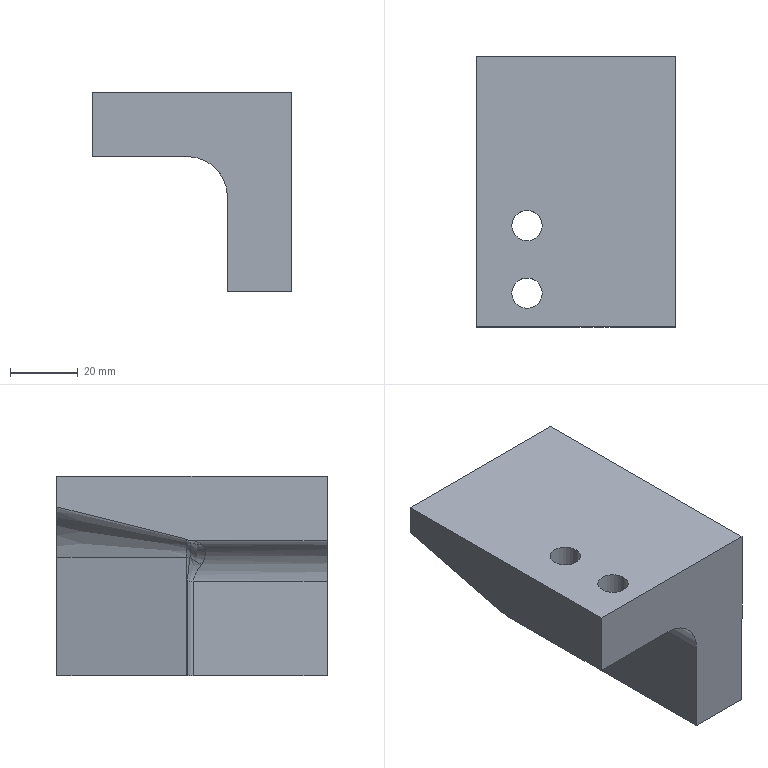Part | 1 solid | 30 faces | box 59 x 80 x 59 mm | volume 130851 mm3 | cylinder 13 | plane 12 | spline 4 | cone 1 | commonest cylinder face diameters 9 x4 15 x4 4 x2 10 x2 24 x1
STEP:
#1=CARTESIAN_POINT('',(-105.5,-10.,19.));
#2=VERTEX_POINT('',#1);
#3=CARTESIAN_POINT('',(-120.5,-10.,19.));
#4=VERTEX_POINT('',#3);
#5=CARTESIAN_POINT('',(-113.,-10.,19.));
#6=DIRECTION('',(0.,0.,1.));
#7=DIRECTION('',(1.,0.,0.));
#8=AXIS2_PLACEMENT_3D('',#5,#6,#7);
#9=CIRCLE('',#8,7.5);
#10=EDGE_CURVE('',#2,#4,#9,.T.);
#11=ORIENTED_EDGE('',*,*,#10,.T.);
#12=CARTESIAN_POINT('',(-120.5,-10.,10.));
#13=VERTEX_POINT('',#12);
#14=CARTESIAN_POINT('',(-120.5,-10.,10.));
#15=DIRECTION('',(0.,0.,-1.));
#16=VECTOR('',#15,1000.);
#17=LINE('',#14,#16);
#18=EDGE_CURVE('',#4,#13,#17,.T.);
#19=ORIENTED_EDGE('',*,*,#18,.T.);
#20=CARTESIAN_POINT('',(-105.5,-10.,10.));
#21=VERTEX_POINT('',#20);
#22=CARTESIAN_POINT('',(-113.,-10.,10.));
#23=DIRECTION('',(0.,0.,1.));
#24=DIRECTION('',(1.,0.,0.));
#25=AXIS2_PLACEMENT_3D('',#22,#23,#24);
#26=CIRCLE('',#25,7.5);
#27=EDGE_CURVE('',#21,#13,#26,.T.);
#28=ORIENTED_EDGE('',*,*,#27,.F.);
#29=CARTESIAN_POINT('',(-105.5,-10.,10.));
#30=DIRECTION('',(0.,0.,-1.));
#31=VECTOR('',#30,1000.);
#32=LINE('',#29,#31);
#33=EDGE_CURVE('',#2,#21,#32,.T.);
#34=ORIENTED_EDGE('',*,*,#33,.F.);
#35=EDGE_LOOP('',(#11,#19,#28,#34));
#36=FACE_OUTER_BOUND('',#35,.T.);
#37=CARTESIAN_POINT('',(-113.,-10.,10.));
#38=DIRECTION('',(0.,0.,-1.));
#39=DIRECTION('',(1.,0.,0.));
#40=AXIS2_PLACEMENT_3D('',#37,#38,#39);
#41=CYLINDRICAL_SURFACE('',#40,7.5);
#42=ADVANCED_FACE('',(#36),#41,.F.);
#43=CARTESIAN_POINT('',(-105.5,-30.,19.));
#44=VERTEX_POINT('',#43);
#45=CARTESIAN_POINT('',(-120.5,-30.,19.));
#46=VERTEX_POINT('',#45);
#47=CARTESIAN_POINT('',(-113.,-30.,19.));
#48=DIRECTION('',(0.,0.,1.));
#49=DIRECTION('',(1.,0.,0.));
#50=AXIS2_PLACEMENT_3D('',#47,#48,#49);
#51=CIRCLE('',#50,7.5);
#52=EDGE_CURVE('',#44,#46,#51,.T.);
#53=ORIENTED_EDGE('',*,*,#52,.T.);
#54=CARTESIAN_POINT('',(-120.5,-30.,10.));
#55=VERTEX_POINT('',#54);
#56=CARTESIAN_POINT('',(-120.5,-30.,10.));
#57=DIRECTION('',(0.,0.,-1.));
#58=VECTOR('',#57,1000.);
#59=LINE('',#56,#58);
#60=EDGE_CURVE('',#46,#55,#59,.T.);
#61=ORIENTED_EDGE('',*,*,#60,.T.);
#62=CARTESIAN_POINT('',(-105.5,-30.,10.));
#63=VERTEX_POINT('',#62);
#64=CARTESIAN_POINT('',(-113.,-30.,10.));
#65=DIRECTION('',(0.,0.,1.));
#66=DIRECTION('',(1.,0.,0.));
#67=AXIS2_PLACEMENT_3D('',#64,#65,#66);
#68=CIRCLE('',#67,7.5);
#69=EDGE_CURVE('',#63,#55,#68,.T.);
#70=ORIENTED_EDGE('',*,*,#69,.F.);
#71=CARTESIAN_POINT('',(-105.5,-30.,10.));
#72=DIRECTION('',(0.,0.,-1.));
#73=VECTOR('',#72,1000.);
#74=LINE('',#71,#73);
#75=EDGE_CURVE('',#44,#63,#74,.T.);
#76=ORIENTED_EDGE('',*,*,#75,.F.);
#77=EDGE_LOOP('',(#53,#61,#70,#76));
#78=FACE_OUTER_BOUND('',#77,.T.);
#79=CARTESIAN_POINT('',(-113.,-30.,10.));
#80=DIRECTION('',(0.,0.,-1.));
#81=DIRECTION('',(1.,0.,0.));
#82=AXIS2_PLACEMENT_3D('',#79,#80,#81);
#83=CYLINDRICAL_SURFACE('',#82,7.5);
#84=ADVANCED_FACE('',(#78),#83,.F.);
#85=CARTESIAN_POINT('',(-108.5,-10.,29.));
#86=VERTEX_POINT('',#85);
#87=CARTESIAN_POINT('',(-117.5,-10.,29.));
#88=VERTEX_POINT('',#87);
#89=CARTESIAN_POINT('',(-113.,-10.,29.));
#90=DIRECTION('',(0.,0.,1.));
#91=DIRECTION('',(-1.,0.,0.));
#92=AXIS2_PLACEMENT_3D('',#89,#90,#91);
#93=CIRCLE('',#92,4.5);
#94=EDGE_CURVE('',#86,#88,#93,.T.);
#95=ORIENTED_EDGE('',*,*,#94,.T.);
#96=CARTESIAN_POINT('',(-117.5,-10.,19.));
#97=VERTEX_POINT('',#96);
#98=CARTESIAN_POINT('',(-117.5,-10.,10.));
#99=DIRECTION('',(0.,0.,-1.));
#100=VECTOR('',#99,1000.);
#101=LINE('',#98,#100);
#102=EDGE_CURVE('',#88,#97,#101,.T.);
#103=ORIENTED_EDGE('',*,*,#102,.T.);
#104=CARTESIAN_POINT('',(-108.5,-10.,19.));
#105=VERTEX_POINT('',#104);
#106=CARTESIAN_POINT('',(-113.,-10.,19.));
#107=DIRECTION('',(0.,0.,1.));
#108=DIRECTION('',(1.,0.,0.));
#109=AXIS2_PLACEMENT_3D('',#106,#107,#108);
#110=CIRCLE('',#109,4.5);
#111=EDGE_CURVE('',#105,#97,#110,.T.);
#112=ORIENTED_EDGE('',*,*,#111,.F.);
#113=CARTESIAN_POINT('',(-108.5,-10.,10.));
#114=DIRECTION('',(0.,0.,-1.));
#115=VECTOR('',#114,1000.);
#116=LINE('',#113,#115);
#117=EDGE_CURVE('',#86,#105,#116,.T.);
#118=ORIENTED_EDGE('',*,*,#117,.F.);
#119=EDGE_LOOP('',(#95,#103,#112,#118));
#120=FACE_OUTER_BOUND('',#119,.T.);
#121=CARTESIAN_POINT('',(-113.,-10.,10.));
#122=DIRECTION('',(0.,0.,-1.));
#123=DIRECTION('',(1.,0.,0.));
#124=AXIS2_PLACEMENT_3D('',#121,#122,#123);
#125=CYLINDRICAL_SURFACE('',#124,4.5);
#126=ADVANCED_FACE('',(#120),#125,.F.);
#127=CARTESIAN_POINT('',(-108.5,-30.,29.));
#128=VERTEX_POINT('',#127);
#129=CARTESIAN_POINT('',(-117.5,-30.,29.));
#130=VERTEX_POINT('',#129);
#131=CARTESIAN_POINT('',(-113.,-30.,29.));
#132=DIRECTION('',(0.,0.,1.));
#133=DIRECTION('',(-1.,0.,0.));
#134=AXIS2_PLACEMENT_3D('',#131,#132,#133);
#135=CIRCLE('',#134,4.5);
#136=EDGE_CURVE('',#128,#130,#135,.T.);
#137=ORIENTED_EDGE('',*,*,#136,.T.);
#138=CARTESIAN_POINT('',(-117.5,-30.,19.));
#139=VERTEX_POINT('',#138);
#140=CARTESIAN_POINT('',(-117.5,-30.,10.));
#141=DIRECTION('',(0.,0.,-1.));
#142=VECTOR('',#141,1000.);
#143=LINE('',#140,#142);
#144=EDGE_CURVE('',#130,#139,#143,.T.);
#145=ORIENTED_EDGE('',*,*,#144,.T.);
#146=CARTESIAN_POINT('',(-108.5,-30.,19.));
#147=VERTEX_POINT('',#146);
#148=CARTESIAN_POINT('',(-113.,-30.,19.));
#149=DIRECTION('',(0.,0.,1.));
#150=DIRECTION('',(1.,0.,0.));
#151=AXIS2_PLACEMENT_3D('',#148,#149,#150);
#152=CIRCLE('',#151,4.5);
#153=EDGE_CURVE('',#147,#139,#152,.T.);
#154=ORIENTED_EDGE('',*,*,#153,.F.);
#155=CARTESIAN_POINT('',(-108.5,-30.,10.));
#156=DIRECTION('',(0.,0.,-1.));
#157=VECTOR('',#156,1000.);
#158=LINE('',#155,#157);
#159=EDGE_CURVE('',#128,#147,#158,.T.);
#160=ORIENTED_EDGE('',*,*,#159,.F.);
#161=EDGE_LOOP('',(#137,#145,#154,#160));
#162=FACE_OUTER_BOUND('',#161,.T.);
#163=CARTESIAN_POINT('',(-113.,-30.,10.));
#164=DIRECTION('',(0.,0.,-1.));
#165=DIRECTION('',(1.,0.,0.));
#166=AXIS2_PLACEMENT_3D('',#163,#164,#165);
#167=CYLINDRICAL_SURFACE('',#166,4.5);
#168=ADVANCED_FACE('',(#162),#167,.F.);
#169=CARTESIAN_POINT('',(-69.,40.,29.));
#170=VERTEX_POINT('',#169);
#171=CARTESIAN_POINT('',(-69.,40.,-30.));
#172=VERTEX_POINT('',#171);
#173=CARTESIAN_POINT('',(-69.,40.,-30.));
#174=DIRECTION('',(0.,0.,-1.));
#175=VECTOR('',#174,1000.);
#176=LINE('',#173,#175);
#177=EDGE_CURVE('',#170,#172,#176,.T.);
#178=ORIENTED_EDGE('',*,*,#177,.T.);
#179=CARTESIAN_POINT('',(-78.,40.,-30.));
#180=VERTEX_POINT('',#179);
#181=CARTESIAN_POINT('',(-88.,40.,-30.));
#182=DIRECTION('',(1.,0.,0.));
#183=VECTOR('',#182,1000.);
#184=LINE('',#181,#183);
#185=EDGE_CURVE('',#180,#172,#184,.T.);
#186=ORIENTED_EDGE('',*,*,#185,.F.);
#187=CARTESIAN_POINT('',(-78.,40.,5.));
#188=VERTEX_POINT('',#187);
#189=CARTESIAN_POINT('',(-78.,40.,5.));
#190=DIRECTION('',(0.,0.,-1.));
#191=VECTOR('',#190,1000.);
#192=LINE('',#189,#191);
#193=EDGE_CURVE('',#188,#180,#192,.T.);
#194=ORIENTED_EDGE('',*,*,#193,.F.);
#195=CARTESIAN_POINT('',(-93.,40.,20.));
#196=VERTEX_POINT('',#195);
#197=CARTESIAN_POINT('',(-93.,40.,5.));
#198=DIRECTION('',(0.,1.,0.));
#199=DIRECTION('',(0.,0.,1.));
#200=AXIS2_PLACEMENT_3D('',#197,#198,#199);
#201=CIRCLE('',#200,15.);
#202=EDGE_CURVE('',#196,#188,#201,.T.);
#203=ORIENTED_EDGE('',*,*,#202,.F.);
#204=CARTESIAN_POINT('',(-128.,40.,20.));
#205=VERTEX_POINT('',#204);
#206=CARTESIAN_POINT('',(-133.,40.,20.));
#207=DIRECTION('',(1.,0.,0.));
#208=VECTOR('',#207,1000.);
#209=LINE('',#206,#208);
#210=EDGE_CURVE('',#205,#196,#209,.T.);
#211=ORIENTED_EDGE('',*,*,#210,.F.);
#212=CARTESIAN_POINT('',(-128.,40.,29.));
#213=VERTEX_POINT('',#212);
#214=CARTESIAN_POINT('',(-128.,40.,30.));
#215=DIRECTION('',(0.,0.,-1.));
#216=VECTOR('',#215,1000.);
#217=LINE('',#214,#216);
#218=EDGE_CURVE('',#213,#205,#217,.T.);
#219=ORIENTED_EDGE('',*,*,#218,.F.);
#220=CARTESIAN_POINT('',(-68.,40.,29.));
#221=DIRECTION('',(1.,0.,0.));
#222=VECTOR('',#221,1000.);
#223=LINE('',#220,#222);
#224=EDGE_CURVE('',#213,#170,#223,.T.);
#225=ORIENTED_EDGE('',*,*,#224,.T.);
#226=EDGE_LOOP('',(#178,#186,#194,#203,#211,#219,#225));
#227=FACE_OUTER_BOUND('',#226,.T.);
#228=CARTESIAN_POINT('',(-100.,40.,-2.));
#229=DIRECTION('',(0.,-1.,0.));
#230=DIRECTION('',(0.,0.,-1.));
#231=AXIS2_PLACEMENT_3D('',#228,#229,#230);
#232=PLANE('',#231);
#233=ADVANCED_FACE('',(#227),#232,.F.);
#234=CARTESIAN_POINT('',(-69.,-40.,29.));
#235=VERTEX_POINT('',#234);
#236=CARTESIAN_POINT('',(-128.,-40.,29.));
#237=VERTEX_POINT('',#236);
#238=CARTESIAN_POINT('',(-68.,-40.,29.));
#239=DIRECTION('',(-1.,0.,0.));
#240=VECTOR('',#239,1000.);
#241=LINE('',#238,#240);
#242=EDGE_CURVE('',#235,#237,#241,.T.);
#243=ORIENTED_EDGE('',*,*,#242,.T.);
#244=CARTESIAN_POINT('',(-128.,-40.,10.));
#245=VERTEX_POINT('',#244);
#246=CARTESIAN_POINT('',(-128.,-40.,30.));
#247=DIRECTION('',(0.,0.,-1.));
#248=VECTOR('',#247,1000.);
#249=LINE('',#246,#248);
#250=EDGE_CURVE('',#237,#245,#249,.T.);
#251=ORIENTED_EDGE('',*,*,#250,.T.);
#252=CARTESIAN_POINT('',(-100.,-40.,10.));
#253=VERTEX_POINT('',#252);
#254=CARTESIAN_POINT('',(-128.,-40.,10.));
#255=DIRECTION('',(1.,0.,0.));
#256=VECTOR('',#255,1000.);
#257=LINE('',#254,#256);
#258=EDGE_CURVE('',#245,#253,#257,.T.);
#259=ORIENTED_EDGE('',*,*,#258,.T.);
#260=CARTESIAN_POINT('',(-88.,-40.,-2.));
#261=VERTEX_POINT('',#260);
#262=CARTESIAN_POINT('',(-100.,-40.,-2.));
#263=DIRECTION('',(0.,1.,0.));
#264=DIRECTION('',(0.,0.,-1.));
#265=AXIS2_PLACEMENT_3D('',#262,#263,#264);
#266=CIRCLE('',#265,12.);
#267=EDGE_CURVE('',#253,#261,#266,.T.);
#268=ORIENTED_EDGE('',*,*,#267,.T.);
#269=CARTESIAN_POINT('',(-88.,-40.,-30.));
#270=VERTEX_POINT('',#269);
#271=CARTESIAN_POINT('',(-88.,-40.,-2.));
#272=DIRECTION('',(0.,0.,-1.));
#273=VECTOR('',#272,1000.);
#274=LINE('',#271,#273);
#275=EDGE_CURVE('',#261,#270,#274,.T.);
#276=ORIENTED_EDGE('',*,*,#275,.T.);
#277=CARTESIAN_POINT('',(-69.,-40.,-30.));
#278=VERTEX_POINT('',#277);
#279=CARTESIAN_POINT('',(-88.,-40.,-30.));
#280=DIRECTION('',(1.,0.,0.));
#281=VECTOR('',#280,1000.);
#282=LINE('',#279,#281);
#283=EDGE_CURVE('',#270,#278,#282,.T.);
#284=ORIENTED_EDGE('',*,*,#283,.T.);
#285=CARTESIAN_POINT('',(-69.,-40.,-30.));
#286=DIRECTION('',(0.,0.,1.));
#287=VECTOR('',#286,1000.);
#288=LINE('',#285,#287);
#289=EDGE_CURVE('',#278,#235,#288,.T.);
#290=ORIENTED_EDGE('',*,*,#289,.T.);
#291=EDGE_LOOP('',(#243,#251,#259,#268,#276,#284,#290));
#292=FACE_OUTER_BOUND('',#291,.T.);
#293=CARTESIAN_POINT('',(-100.,-40.,-2.));
#294=DIRECTION('',(0.,-1.,0.));
#295=DIRECTION('',(0.,0.,-1.));
#296=AXIS2_PLACEMENT_3D('',#293,#294,#295);
#297=PLANE('',#296);
#298=ADVANCED_FACE('',(#292),#297,.T.);
#299=CARTESIAN_POINT('',(-87.621,1.515,-30.));
#300=VERTEX_POINT('',#299);
#301=CARTESIAN_POINT('',(-87.687,1.303,-30.));
#302=VERTEX_POINT('',#301);
#303=CARTESIAN_POINT('',(-89.562,2.,-30.));
#304=DIRECTION('',(0.,0.,-1.));
#305=DIRECTION('',(-1.,0.,0.));
#306=AXIS2_PLACEMENT_3D('',#303,#304,#305);
#307=CIRCLE('',#306,2.);
#308=EDGE_CURVE('',#300,#302,#307,.T.);
#309=ORIENTED_EDGE('',*,*,#308,.F.);
#310=CARTESIAN_POINT('',(-78.,40.,-30.));
#311=DIRECTION('',(-0.2425,-0.9701,0.));
#312=VECTOR('',#311,1000.);
#313=LINE('',#310,#312);
#314=EDGE_CURVE('',#180,#300,#313,.T.);
#315=ORIENTED_EDGE('',*,*,#314,.F.);
#316=ORIENTED_EDGE('',*,*,#185,.T.);
#317=CARTESIAN_POINT('',(-69.,40.,-30.));
#318=DIRECTION('',(0.,-1.,0.));
#319=VECTOR('',#318,1000.);
#320=LINE('',#317,#319);
#321=EDGE_CURVE('',#172,#278,#320,.T.);
#322=ORIENTED_EDGE('',*,*,#321,.T.);
#323=ORIENTED_EDGE('',*,*,#283,.F.);
#324=CARTESIAN_POINT('',(-88.,-0.4384,-30.));
#325=VERTEX_POINT('',#324);
#326=CARTESIAN_POINT('',(-88.,40.,-30.));
#327=DIRECTION('',(0.,-1.,0.));
#328=VECTOR('',#327,1000.);
#329=LINE('',#326,#328);
#330=EDGE_CURVE('',#325,#270,#329,.T.);
#331=ORIENTED_EDGE('',*,*,#330,.F.);
#332=CARTESIAN_POINT('',(-83.,-0.4384,-30.));
#333=DIRECTION('',(0.,0.,1.));
#334=DIRECTION('',(-1.,0.,0.));
#335=AXIS2_PLACEMENT_3D('',#332,#333,#334);
#336=CIRCLE('',#335,5.);
#337=EDGE_CURVE('',#302,#325,#336,.T.);
#338=ORIENTED_EDGE('',*,*,#337,.F.);
#339=EDGE_LOOP('',(#309,#315,#316,#322,#323,#331,#338));
#340=FACE_OUTER_BOUND('',#339,.T.);
#341=CARTESIAN_POINT('',(-88.,40.,-30.));
#342=DIRECTION('',(0.,0.,1.));
#343=DIRECTION('',(-1.,0.,0.));
#344=AXIS2_PLACEMENT_3D('',#341,#342,#343);
#345=PLANE('',#344);
#346=ADVANCED_FACE('',(#340),#345,.F.);
#347=ORIENTED_EDGE('',*,*,#94,.F.);
#348=CARTESIAN_POINT('',(-113.,-10.,29.));
#349=DIRECTION('',(0.,0.,1.));
#350=DIRECTION('',(-1.,0.,0.));
#351=AXIS2_PLACEMENT_3D('',#348,#349,#350);
#352=CIRCLE('',#351,4.5);
#353=EDGE_CURVE('',#88,#86,#352,.T.);
#354=ORIENTED_EDGE('',*,*,#353,.F.);
#355=EDGE_LOOP('',(#347,#354));
#356=FACE_BOUND('',#355,.T.);
#357=ORIENTED_EDGE('',*,*,#136,.F.);
#358=CARTESIAN_POINT('',(-113.,-30.,29.));
#359=DIRECTION('',(0.,0.,1.));
#360=DIRECTION('',(-1.,0.,0.));
#361=AXIS2_PLACEMENT_3D('',#358,#359,#360);
#362=CIRCLE('',#361,4.5);
#363=EDGE_CURVE('',#130,#128,#362,.T.);
#364=ORIENTED_EDGE('',*,*,#363,.F.);
#365=EDGE_LOOP('',(#357,#364));
#366=FACE_BOUND('',#365,.T.);
#367=ORIENTED_EDGE('',*,*,#224,.F.);
#368=CARTESIAN_POINT('',(-128.,40.,29.));
#369=DIRECTION('',(0.,1.,0.));
#370=VECTOR('',#369,1000.);
#371=LINE('',#368,#370);
#372=EDGE_CURVE('',#237,#213,#371,.T.);
#373=ORIENTED_EDGE('',*,*,#372,.F.);
#374=ORIENTED_EDGE('',*,*,#242,.F.);
#375=CARTESIAN_POINT('',(-69.,40.,29.));
#376=DIRECTION('',(0.,1.,0.));
#377=VECTOR('',#376,1000.);
#378=LINE('',#375,#377);
#379=EDGE_CURVE('',#235,#170,#378,.T.);
#380=ORIENTED_EDGE('',*,*,#379,.T.);
#381=EDGE_LOOP('',(#367,#373,#374,#380));
#382=FACE_OUTER_BOUND('',#381,.T.);
#383=CARTESIAN_POINT('',(-98.,0.,29.));
#384=DIRECTION('',(0.,0.,1.));
#385=DIRECTION('',(-1.,0.,0.));
#386=AXIS2_PLACEMENT_3D('',#383,#384,#385);
#387=PLANE('',#386);
#388=ADVANCED_FACE('',(#356,#366,#382),#387,.T.);
#389=CARTESIAN_POINT('',(-128.,-0.4384,10.));
#390=VERTEX_POINT('',#389);
#391=CARTESIAN_POINT('',(-128.,40.,10.));
#392=DIRECTION('',(0.,-1.,0.));
#393=VECTOR('',#392,1000.);
#394=LINE('',#391,#393);
#395=EDGE_CURVE('',#390,#245,#394,.T.);
#396=ORIENTED_EDGE('',*,*,#395,.T.);
#397=ORIENTED_EDGE('',*,*,#250,.F.);
#398=ORIENTED_EDGE('',*,*,#372,.T.);
#399=ORIENTED_EDGE('',*,*,#218,.T.);
#400=CARTESIAN_POINT('',(-128.,1.515,10.379));
#401=VERTEX_POINT('',#400);
#402=CARTESIAN_POINT('',(-128.,40.,20.));
#403=DIRECTION('',(0.,0.9701,0.2425));
#404=VECTOR('',#403,1000.);
#405=LINE('',#402,#404);
#406=EDGE_CURVE('',#401,#205,#405,.T.);
#407=ORIENTED_EDGE('',*,*,#406,.F.);
#408=CARTESIAN_POINT('',(-128.,1.303,10.313));
#409=VERTEX_POINT('',#408);
#410=CARTESIAN_POINT('',(-128.,2.,8.438));
#411=DIRECTION('',(-1.,0.,0.));
#412=DIRECTION('',(0.,0.,1.));
#413=AXIS2_PLACEMENT_3D('',#410,#411,#412);
#414=CIRCLE('',#413,2.);
#415=EDGE_CURVE('',#409,#401,#414,.T.);
#416=ORIENTED_EDGE('',*,*,#415,.F.);
#417=CARTESIAN_POINT('',(-128.,-0.4384,15.));
#418=DIRECTION('',(1.,0.,0.));
#419=DIRECTION('',(0.,0.,1.));
#420=AXIS2_PLACEMENT_3D('',#417,#418,#419);
#421=CIRCLE('',#420,5.);
#422=EDGE_CURVE('',#390,#409,#421,.T.);
#423=ORIENTED_EDGE('',*,*,#422,.F.);
#424=EDGE_LOOP('',(#396,#397,#398,#399,#407,#416,#423));
#425=FACE_OUTER_BOUND('',#424,.T.);
#426=CARTESIAN_POINT('',(-128.,40.,30.));
#427=DIRECTION('',(1.,0.,0.));
#428=DIRECTION('',(0.,0.,1.));
#429=AXIS2_PLACEMENT_3D('',#426,#427,#428);
#430=PLANE('',#429);
#431=ADVANCED_FACE('',(#425),#430,.F.);
#432=ORIENTED_EDGE('',*,*,#144,.F.);
#433=ORIENTED_EDGE('',*,*,#363,.T.);
#434=ORIENTED_EDGE('',*,*,#159,.T.);
#435=CARTESIAN_POINT('',(-113.,-30.,19.));
#436=DIRECTION('',(0.,0.,1.));
#437=DIRECTION('',(1.,0.,0.));
#438=AXIS2_PLACEMENT_3D('',#435,#436,#437);
#439=CIRCLE('',#438,4.5);
#440=EDGE_CURVE('',#139,#147,#439,.T.);
#441=ORIENTED_EDGE('',*,*,#440,.F.);
#442=EDGE_LOOP('',(#432,#433,#434,#441));
#443=FACE_OUTER_BOUND('',#442,.T.);
#444=CARTESIAN_POINT('',(-113.,-30.,10.));
#445=DIRECTION('',(0.,0.,-1.));
#446=DIRECTION('',(1.,0.,0.));
#447=AXIS2_PLACEMENT_3D('',#444,#445,#446);
#448=CYLINDRICAL_SURFACE('',#447,4.5);
#449=ADVANCED_FACE('',(#443),#448,.F.);
#450=ORIENTED_EDGE('',*,*,#102,.F.);
#451=ORIENTED_EDGE('',*,*,#353,.T.);
#452=ORIENTED_EDGE('',*,*,#117,.T.);
#453=CARTESIAN_POINT('',(-113.,-10.,19.));
#454=DIRECTION('',(0.,0.,1.));
#455=DIRECTION('',(1.,0.,0.));
#456=AXIS2_PLACEMENT_3D('',#453,#454,#455);
#457=CIRCLE('',#456,4.5);
#458=EDGE_CURVE('',#97,#105,#457,.T.);
#459=ORIENTED_EDGE('',*,*,#458,.F.);
#460=EDGE_LOOP('',(#450,#451,#452,#459));
#461=FACE_OUTER_BOUND('',#460,.T.);
#462=CARTESIAN_POINT('',(-113.,-10.,10.));
#463=DIRECTION('',(0.,0.,-1.));
#464=DIRECTION('',(1.,0.,0.));
#465=AXIS2_PLACEMENT_3D('',#462,#463,#464);
#466=CYLINDRICAL_SURFACE('',#465,4.5);
#467=ADVANCED_FACE('',(#461),#466,.F.);
#468=CARTESIAN_POINT('',(-88.,-0.4384,-2.));
#469=VERTEX_POINT('',#468);
#470=CARTESIAN_POINT('',(-88.,40.,-2.));
#471=DIRECTION('',(0.,-1.,0.));
#472=VECTOR('',#471,1000.);
#473=LINE('',#470,#472);
#474=EDGE_CURVE('',#469,#261,#473,.T.);
#475=ORIENTED_EDGE('',*,*,#474,.T.);
#476=ORIENTED_EDGE('',*,*,#267,.F.);
#477=CARTESIAN_POINT('',(-100.,-0.4384,10.));
#478=VERTEX_POINT('',#477);
#479=CARTESIAN_POINT('',(-100.,40.,10.));
#480=DIRECTION('',(0.,-1.,0.));
#481=VECTOR('',#480,1000.);
#482=LINE('',#479,#481);
#483=EDGE_CURVE('',#478,#253,#482,.T.);
#484=ORIENTED_EDGE('',*,*,#483,.F.);
#485=CARTESIAN_POINT('',(-95.059,-2.844,8.935));
#486=VERTEX_POINT('',#485);
#487=CARTESIAN_POINT('',(-95.059,-2.844,8.935));
#488=CARTESIAN_POINT('',(-95.512,-2.541,9.14));
#489=CARTESIAN_POINT('',(-95.939,-2.252,9.3));
#490=CARTESIAN_POINT('',(-96.774,-1.707,9.566));
#491=CARTESIAN_POINT('',(-97.183,-1.449,9.672));
#492=CARTESIAN_POINT('',(-98.391,-0.7712,9.92));
#493=CARTESIAN_POINT('',(-99.177,-0.4384,10.));
#494=CARTESIAN_POINT('',(-100.,-0.4384,10.));
#495=B_SPLINE_CURVE_WITH_KNOTS('',3,(#487,#488,#489,#490,#491,#492,#493,#494),.UNSPECIFIED.,.F.,.F.,(4,2,2,4),(0.,0.25,0.5,1.),.UNSPECIFIED.);
#496=EDGE_CURVE('',#486,#478,#495,.T.);
#497=ORIENTED_EDGE('',*,*,#496,.F.);
#498=CARTESIAN_POINT('',(-89.065,-2.844,2.941));
#499=VERTEX_POINT('',#498);
#500=CARTESIAN_POINT('',(-89.065,-2.844,2.941));
#501=CARTESIAN_POINT('',(-89.199,-3.042,3.238));
#502=CARTESIAN_POINT('',(-89.35,-3.21,3.54));
#503=CARTESIAN_POINT('',(-89.69,-3.493,4.15));
#504=CARTESIAN_POINT('',(-89.88,-3.61,4.46));
#505=CARTESIAN_POINT('',(-90.295,-3.792,5.067));
#506=CARTESIAN_POINT('',(-90.517,-3.857,5.363));
#507=CARTESIAN_POINT('',(-90.993,-3.944,5.938));
#508=CARTESIAN_POINT('',(-91.245,-3.966,6.216));
#509=CARTESIAN_POINT('',(-91.784,-3.966,6.754));
#510=CARTESIAN_POINT('',(-92.062,-3.944,7.007));
#511=CARTESIAN_POINT('',(-92.638,-3.857,7.483));
#512=CARTESIAN_POINT('',(-92.934,-3.791,7.706));
#513=CARTESIAN_POINT('',(-93.544,-3.608,8.122));
#514=CARTESIAN_POINT('',(-93.851,-3.492,8.311));
#515=CARTESIAN_POINT('',(-94.46,-3.209,8.65));
#516=CARTESIAN_POINT('',(-94.762,-3.042,8.801));
#517=CARTESIAN_POINT('',(-95.059,-2.844,8.935));
#518=B_SPLINE_CURVE_WITH_KNOTS('',3,(#500,#501,#502,#503,#504,#505,#506,#507,#508,#509,#510,#511,#512,#513,#514,#515,#516,#517),.UNSPECIFIED.,.F.,.F.,(4,2,2,2,2,2,2,2,4),(0.,0.00113,0.00226,0.00339,0.00452,0.00565,0.00678,0.00791,0.00904),.UNSPECIFIED.);
#519=EDGE_CURVE('',#499,#486,#518,.T.);
#520=ORIENTED_EDGE('',*,*,#519,.F.);
#521=CARTESIAN_POINT('',(-88.,-0.4384,-2.));
#522=CARTESIAN_POINT('',(-88.,-0.4384,-1.518));
#523=CARTESIAN_POINT('',(-88.028,-0.5512,-1.061));
#524=CARTESIAN_POINT('',(-88.131,-0.8956,-0.1754));
#525=CARTESIAN_POINT('',(-88.204,-1.12,0.2431));
#526=CARTESIAN_POINT('',(-88.386,-1.591,1.047));
#527=CARTESIAN_POINT('',(-88.495,-1.841,1.434));
#528=CARTESIAN_POINT('',(-88.75,-2.343,2.196));
#529=CARTESIAN_POINT('',(-88.897,-2.596,2.57));
#530=CARTESIAN_POINT('',(-89.065,-2.844,2.941));
#531=B_SPLINE_CURVE_WITH_KNOTS('',3,(#521,#522,#523,#524,#525,#526,#527,#528,#529,#530),.UNSPECIFIED.,.F.,.F.,(4,2,2,2,4),(0.,0.001413,0.002826,0.004239,0.005652),.UNSPECIFIED.);
#532=EDGE_CURVE('',#469,#499,#531,.T.);
#533=ORIENTED_EDGE('',*,*,#532,.F.);
#534=EDGE_LOOP('',(#475,#476,#484,#497,#520,#533));
#535=FACE_OUTER_BOUND('',#534,.T.);
#536=CARTESIAN_POINT('',(-100.,40.,-2.));
#537=DIRECTION('',(0.,-1.,0.));
#538=DIRECTION('',(0.,0.,-1.));
#539=AXIS2_PLACEMENT_3D('',#536,#537,#538);
#540=CYLINDRICAL_SURFACE('',#539,12.);
#541=ADVANCED_FACE('',(#535),#540,.F.);
#542=ORIENTED_EDGE('',*,*,#27,.T.);
#543=CARTESIAN_POINT('',(-113.,-10.,10.));
#544=DIRECTION('',(0.,0.,1.));
#545=DIRECTION('',(1.,0.,0.));
#546=AXIS2_PLACEMENT_3D('',#543,#544,#545);
#547=CIRCLE('',#546,7.5);
#548=EDGE_CURVE('',#13,#21,#547,.T.);
#549=ORIENTED_EDGE('',*,*,#548,.T.);
#550=EDGE_LOOP('',(#542,#549));
#551=FACE_BOUND('',#550,.T.);
#552=ORIENTED_EDGE('',*,*,#69,.T.);
#553=CARTESIAN_POINT('',(-113.,-30.,10.));
#554=DIRECTION('',(0.,0.,1.));
#555=DIRECTION('',(1.,0.,0.));
#556=AXIS2_PLACEMENT_3D('',#553,#554,#555);
#557=CIRCLE('',#556,7.5);
#558=EDGE_CURVE('',#55,#63,#557,.T.);
#559=ORIENTED_EDGE('',*,*,#558,.T.);
#560=EDGE_LOOP('',(#552,#559));
#561=FACE_BOUND('',#560,.T.);
#562=ORIENTED_EDGE('',*,*,#483,.T.);
#563=ORIENTED_EDGE('',*,*,#258,.F.);
#564=ORIENTED_EDGE('',*,*,#395,.F.);
#565=CARTESIAN_POINT('',(-128.,-0.4384,10.));
#566=DIRECTION('',(-1.,0.,0.));
#567=VECTOR('',#566,1000.);
#568=LINE('',#565,#567);
#569=EDGE_CURVE('',#478,#390,#568,.T.);
#570=ORIENTED_EDGE('',*,*,#569,.F.);
#571=EDGE_LOOP('',(#562,#563,#564,#570));
#572=FACE_OUTER_BOUND('',#571,.T.);
#573=CARTESIAN_POINT('',(-128.,40.,10.));
#574=DIRECTION('',(0.,0.,1.));
#575=DIRECTION('',(-1.,0.,0.));
#576=AXIS2_PLACEMENT_3D('',#573,#574,#575);
#577=PLANE('',#576);
#578=ADVANCED_FACE('',(#551,#561,#572),#577,.F.);
#579=ORIENTED_EDGE('',*,*,#330,.T.);
#580=ORIENTED_EDGE('',*,*,#275,.F.);
#581=ORIENTED_EDGE('',*,*,#474,.F.);
#582=CARTESIAN_POINT('',(-88.,-0.4384,-2.));
#583=DIRECTION('',(0.,0.,1.));
#584=VECTOR('',#583,1000.);
#585=LINE('',#582,#584);
#586=EDGE_CURVE('',#325,#469,#585,.T.);
#587=ORIENTED_EDGE('',*,*,#586,.F.);
#588=EDGE_LOOP('',(#579,#580,#581,#587));
#589=FACE_OUTER_BOUND('',#588,.T.);
#590=CARTESIAN_POINT('',(-88.,40.,-2.));
#591=DIRECTION('',(1.,0.,0.));
#592=DIRECTION('',(0.,0.,1.));
#593=AXIS2_PLACEMENT_3D('',#590,#591,#592);
#594=PLANE('',#593);
#595=ADVANCED_FACE('',(#589),#594,.F.);
#596=ORIENTED_EDGE('',*,*,#406,.T.);
#597=ORIENTED_EDGE('',*,*,#210,.T.);
#598=CARTESIAN_POINT('',(-93.,1.515,10.379));
#599=VERTEX_POINT('',#598);
#600=CARTESIAN_POINT('',(-93.,40.,20.));
#601=DIRECTION('',(0.,-0.9701,-0.2425));
#602=VECTOR('',#601,1000.);
#603=LINE('',#600,#602);
#604=EDGE_CURVE('',#196,#599,#603,.T.);
#605=ORIENTED_EDGE('',*,*,#604,.T.);
#606=CARTESIAN_POINT('',(-93.,1.515,10.379));
#607=DIRECTION('',(1.,0.,0.));
#608=VECTOR('',#607,1000.);
#609=LINE('',#606,#608);
#610=EDGE_CURVE('',#401,#599,#609,.T.);
#611=ORIENTED_EDGE('',*,*,#610,.F.);
#612=EDGE_LOOP('',(#596,#597,#605,#611));
#613=FACE_OUTER_BOUND('',#612,.T.);
#614=CARTESIAN_POINT('',(-133.,40.,20.));
#615=DIRECTION('',(0.,0.2425,-0.9701));
#616=DIRECTION('',(0.,0.9701,0.2425));
#617=AXIS2_PLACEMENT_3D('',#614,#615,#616);
#618=PLANE('',#617);
#619=ADVANCED_FACE('',(#613),#618,.T.);
#620=ORIENTED_EDGE('',*,*,#604,.F.);
#621=ORIENTED_EDGE('',*,*,#202,.T.);
#622=CARTESIAN_POINT('',(-87.621,1.515,5.));
#623=VERTEX_POINT('',#622);
#624=CARTESIAN_POINT('',(-78.,40.,5.));
#625=DIRECTION('',(-0.2425,-0.9701,0.));
#626=VECTOR('',#625,1000.);
#627=LINE('',#624,#626);
#628=EDGE_CURVE('',#188,#623,#627,.T.);
#629=ORIENTED_EDGE('',*,*,#628,.T.);
#630=CARTESIAN_POINT('',(-93.,1.515,10.379));
#631=CARTESIAN_POINT('',(-92.296,1.515,10.379));
#632=CARTESIAN_POINT('',(-91.592,1.515,10.239));
#633=CARTESIAN_POINT('',(-90.291,1.515,9.7));
#634=CARTESIAN_POINT('',(-89.695,1.515,9.301));
#635=CARTESIAN_POINT('',(-88.699,1.515,8.305));
#636=CARTESIAN_POINT('',(-88.3,1.515,7.709));
#637=CARTESIAN_POINT('',(-87.761,1.515,6.408));
#638=CARTESIAN_POINT('',(-87.621,1.515,5.704));
#639=CARTESIAN_POINT('',(-87.621,1.515,5.));
#640=B_SPLINE_CURVE_WITH_KNOTS('',3,(#630,#631,#632,#633,#634,#635,#636,#637,#638,#639),.UNSPECIFIED.,.F.,.F.,(4,2,2,2,4),(0.,0.25,0.5,0.75,1.),.UNSPECIFIED.);
#641=EDGE_CURVE('',#599,#623,#640,.T.);
#642=ORIENTED_EDGE('',*,*,#641,.F.);
#643=EDGE_LOOP('',(#620,#621,#629,#642));
#644=FACE_OUTER_BOUND('',#643,.T.);
#645=CARTESIAN_POINT('',(-93.,40.,5.));
#646=DIRECTION('',(0.,1.,0.));
#647=DIRECTION('',(0.,0.,1.));
#648=AXIS2_PLACEMENT_3D('',#645,#646,#647);
#649=CONICAL_SURFACE('',#648,15.,0.245);
#650=ADVANCED_FACE('',(#644),#649,.F.);
#651=ORIENTED_EDGE('',*,*,#628,.F.);
#652=ORIENTED_EDGE('',*,*,#193,.T.);
#653=ORIENTED_EDGE('',*,*,#314,.T.);
#654=CARTESIAN_POINT('',(-87.621,1.515,-2.));
#655=DIRECTION('',(0.,0.,-1.));
#656=VECTOR('',#655,1000.);
#657=LINE('',#654,#656);
#658=EDGE_CURVE('',#623,#300,#657,.T.);
#659=ORIENTED_EDGE('',*,*,#658,.F.);
#660=EDGE_LOOP('',(#651,#652,#653,#659));
#661=FACE_OUTER_BOUND('',#660,.T.);
#662=CARTESIAN_POINT('',(-78.,40.,5.));
#663=DIRECTION('',(-0.9701,0.2425,0.));
#664=DIRECTION('',(0.2425,0.9701,0.));
#665=AXIS2_PLACEMENT_3D('',#662,#663,#664);
#666=PLANE('',#665);
#667=ADVANCED_FACE('',(#661),#666,.T.);
#668=ORIENTED_EDGE('',*,*,#153,.T.);
#669=ORIENTED_EDGE('',*,*,#440,.T.);
#670=EDGE_LOOP('',(#668,#669));
#671=FACE_BOUND('',#670,.T.);
#672=ORIENTED_EDGE('',*,*,#52,.F.);
#673=CARTESIAN_POINT('',(-113.,-30.,19.));
#674=DIRECTION('',(0.,0.,1.));
#675=DIRECTION('',(1.,0.,0.));
#676=AXIS2_PLACEMENT_3D('',#673,#674,#675);
#677=CIRCLE('',#676,7.5);
#678=EDGE_CURVE('',#46,#44,#677,.T.);
#679=ORIENTED_EDGE('',*,*,#678,.F.);
#680=EDGE_LOOP('',(#672,#679));
#681=FACE_OUTER_BOUND('',#680,.T.);
#682=CARTESIAN_POINT('',(-117.5,-30.,19.));
#683=DIRECTION('',(0.,0.,1.));
#684=DIRECTION('',(-1.,0.,0.));
#685=AXIS2_PLACEMENT_3D('',#682,#683,#684);
#686=PLANE('',#685);
#687=ADVANCED_FACE('',(#671,#681),#686,.F.);
#688=ORIENTED_EDGE('',*,*,#60,.F.);
#689=ORIENTED_EDGE('',*,*,#678,.T.);
#690=ORIENTED_EDGE('',*,*,#75,.T.);
#691=ORIENTED_EDGE('',*,*,#558,.F.);
#692=EDGE_LOOP('',(#688,#689,#690,#691));
#693=FACE_OUTER_BOUND('',#692,.T.);
#694=CARTESIAN_POINT('',(-113.,-30.,10.));
#695=DIRECTION('',(0.,0.,-1.));
#696=DIRECTION('',(1.,0.,0.));
#697=AXIS2_PLACEMENT_3D('',#694,#695,#696);
#698=CYLINDRICAL_SURFACE('',#697,7.5);
#699=ADVANCED_FACE('',(#693),#698,.F.);
#700=ORIENTED_EDGE('',*,*,#111,.T.);
#701=ORIENTED_EDGE('',*,*,#458,.T.);
#702=EDGE_LOOP('',(#700,#701));
#703=FACE_BOUND('',#702,.T.);
#704=ORIENTED_EDGE('',*,*,#10,.F.);
#705=CARTESIAN_POINT('',(-113.,-10.,19.));
#706=DIRECTION('',(0.,0.,1.));
#707=DIRECTION('',(1.,0.,0.));
#708=AXIS2_PLACEMENT_3D('',#705,#706,#707);
#709=CIRCLE('',#708,7.5);
#710=EDGE_CURVE('',#4,#2,#709,.T.);
#711=ORIENTED_EDGE('',*,*,#710,.F.);
#712=EDGE_LOOP('',(#704,#711));
#713=FACE_OUTER_BOUND('',#712,.T.);
#714=CARTESIAN_POINT('',(-117.5,-10.,19.));
#715=DIRECTION('',(0.,0.,1.));
#716=DIRECTION('',(-1.,0.,0.));
#717=AXIS2_PLACEMENT_3D('',#714,#715,#716);
#718=PLANE('',#717);
#719=ADVANCED_FACE('',(#703,#713),#718,.F.);
#720=ORIENTED_EDGE('',*,*,#18,.F.);
#721=ORIENTED_EDGE('',*,*,#710,.T.);
#722=ORIENTED_EDGE('',*,*,#33,.T.);
#723=ORIENTED_EDGE('',*,*,#548,.F.);
#724=EDGE_LOOP('',(#720,#721,#722,#723));
#725=FACE_OUTER_BOUND('',#724,.T.);
#726=CARTESIAN_POINT('',(-113.,-10.,10.));
#727=DIRECTION('',(0.,0.,-1.));
#728=DIRECTION('',(1.,0.,0.));
#729=AXIS2_PLACEMENT_3D('',#726,#727,#728);
#730=CYLINDRICAL_SURFACE('',#729,7.5);
#731=ADVANCED_FACE('',(#725),#730,.F.);
#732=ORIENTED_EDGE('',*,*,#321,.F.);
#733=ORIENTED_EDGE('',*,*,#177,.F.);
#734=ORIENTED_EDGE('',*,*,#379,.F.);
#735=ORIENTED_EDGE('',*,*,#289,.F.);
#736=EDGE_LOOP('',(#732,#733,#734,#735));
#737=FACE_OUTER_BOUND('',#736,.T.);
#738=CARTESIAN_POINT('',(-69.,0.,0.));
#739=DIRECTION('',(1.,0.,0.));
#740=DIRECTION('',(0.,0.,1.));
#741=AXIS2_PLACEMENT_3D('',#738,#739,#740);
#742=PLANE('',#741);
#743=ADVANCED_FACE('',(#737),#742,.T.);
#744=CARTESIAN_POINT('',(-88.118,0.6161,5.));
#745=VERTEX_POINT('',#744);
#746=CARTESIAN_POINT('',(-87.687,1.303,-2.));
#747=VERTEX_POINT('',#746);
#748=CARTESIAN_POINT('',(-88.118,0.6161,5.));
#749=CARTESIAN_POINT('',(-87.968,0.7719,3.843));
#750=CARTESIAN_POINT('',(-87.862,0.9343,2.683));
#751=CARTESIAN_POINT('',(-87.721,1.202,0.3503));
#752=CARTESIAN_POINT('',(-87.687,1.303,-0.8223));
#753=CARTESIAN_POINT('',(-87.687,1.303,-2.));
#754=B_SPLINE_CURVE_WITH_KNOTS('',3,(#748,#749,#750,#751,#752,#753),.UNSPECIFIED.,.F.,.F.,(4,2,4),(0.,0.003527,0.007055),.UNSPECIFIED.);
#755=EDGE_CURVE('',#745,#747,#754,.T.);
#756=ORIENTED_EDGE('',*,*,#755,.F.);
#757=CARTESIAN_POINT('',(-88.118,0.6161,5.));
#758=CARTESIAN_POINT('',(-87.878,0.866,5.));
#759=CARTESIAN_POINT('',(-87.705,1.179,5.));
#760=CARTESIAN_POINT('',(-87.621,1.515,5.));
#761=B_SPLINE_CURVE_WITH_KNOTS('',3,(#757,#758,#759,#760),.UNSPECIFIED.,.F.,.F.,(4,4),(0.6084,1.),.UNSPECIFIED.);
#762=EDGE_CURVE('',#745,#623,#761,.T.);
#763=ORIENTED_EDGE('',*,*,#762,.T.);
#764=ORIENTED_EDGE('',*,*,#658,.T.);
#765=ORIENTED_EDGE('',*,*,#308,.T.);
#766=CARTESIAN_POINT('',(-87.687,1.303,5.));
#767=DIRECTION('',(0.,0.,-1.));
#768=VECTOR('',#767,1000.);
#769=LINE('',#766,#768);
#770=EDGE_CURVE('',#747,#302,#769,.T.);
#771=ORIENTED_EDGE('',*,*,#770,.F.);
#772=EDGE_LOOP('',(#756,#763,#764,#765,#771));
#773=FACE_OUTER_BOUND('',#772,.T.);
#774=CARTESIAN_POINT('',(-89.562,2.,5.));
#775=DIRECTION('',(0.,0.,1.));
#776=DIRECTION('',(-1.,0.,0.));
#777=AXIS2_PLACEMENT_3D('',#774,#775,#776);
#778=CYLINDRICAL_SURFACE('',#777,2.);
#779=ADVANCED_FACE('',(#773),#778,.F.);
#780=CARTESIAN_POINT('',(-93.,0.6161,9.882));
#781=VERTEX_POINT('',#780);
#782=CARTESIAN_POINT('',(-93.,0.6161,9.882));
#783=CARTESIAN_POINT('',(-93.,0.9996,10.25));
#784=CARTESIAN_POINT('',(-93.,1.515,10.379));
#785=(BOUNDED_CURVE()B_SPLINE_CURVE(2,(#782,#783,#784),.UNSPECIFIED.,.F.,.F.)B_SPLINE_CURVE_WITH_KNOTS((3,3),(0.6045,1.),.UNSPECIFIED.)CURVE()GEOMETRIC_REPRESENTATION_ITEM()RATIONAL_B_SPLINE_CURVE((0.8987,0.9162,1.))REPRESENTATION_ITEM(''));
#786=EDGE_CURVE('',#781,#599,#785,.T.);
#787=ORIENTED_EDGE('',*,*,#786,.T.);
#788=ORIENTED_EDGE('',*,*,#641,.T.);
#789=ORIENTED_EDGE('',*,*,#762,.F.);
#790=CARTESIAN_POINT('',(-93.,0.6161,9.882));
#791=CARTESIAN_POINT('',(-92.855,0.5818,9.849));
#792=CARTESIAN_POINT('',(-92.707,0.5516,9.811));
#793=CARTESIAN_POINT('',(-92.418,0.4986,9.727));
#794=CARTESIAN_POINT('',(-92.274,0.4756,9.68));
#795=CARTESIAN_POINT('',(-91.847,0.4143,9.524));
#796=CARTESIAN_POINT('',(-91.565,0.3836,9.399));
#797=CARTESIAN_POINT('',(-90.755,0.3137,8.967));
#798=CARTESIAN_POINT('',(-90.265,0.2955,8.607));
#799=CARTESIAN_POINT('',(-89.392,0.2955,7.734));
#800=CARTESIAN_POINT('',(-89.033,0.3138,7.244));
#801=CARTESIAN_POINT('',(-88.602,0.3835,6.437));
#802=CARTESIAN_POINT('',(-88.477,0.4141,6.154));
#803=CARTESIAN_POINT('',(-88.321,0.4755,5.726));
#804=CARTESIAN_POINT('',(-88.273,0.4986,5.583));
#805=CARTESIAN_POINT('',(-88.189,0.5516,5.293));
#806=CARTESIAN_POINT('',(-88.151,0.5818,5.145));
#807=CARTESIAN_POINT('',(-88.118,0.6161,5.));
#808=B_SPLINE_CURVE_WITH_KNOTS('',3,(#790,#791,#792,#793,#794,#795,#796,#797,#798,#799,#800,#801,#802,#803,#804,#805,#806,#807),.UNSPECIFIED.,.F.,.F.,(4,2,2,2,2,2,2,2,4),(-0.00000006,0.0004588,0.0009177,0.001835,0.003671,0.005506,0.006424,0.006883,0.007342),.UNSPECIFIED.);
#809=EDGE_CURVE('',#781,#745,#808,.T.);
#810=ORIENTED_EDGE('',*,*,#809,.F.);
#811=EDGE_LOOP('',(#787,#788,#789,#810));
#812=FACE_OUTER_BOUND('',#811,.T.);
#813=CARTESIAN_POINT('',(-93.,1.515,10.379));
#814=CARTESIAN_POINT('',(-92.296,1.515,10.379));
#815=CARTESIAN_POINT('',(-91.592,1.515,10.239));
#816=CARTESIAN_POINT('',(-90.291,1.515,9.7));
#817=CARTESIAN_POINT('',(-89.695,1.515,9.301));
#818=CARTESIAN_POINT('',(-88.699,1.515,8.305));
#819=CARTESIAN_POINT('',(-88.3,1.515,7.709));
#820=CARTESIAN_POINT('',(-87.761,1.515,6.408));
#821=CARTESIAN_POINT('',(-87.621,1.515,5.704));
#822=CARTESIAN_POINT('',(-87.621,1.515,5.));
#823=CARTESIAN_POINT('',(-93.,0.,10.));
#824=CARTESIAN_POINT('',(-92.345,0.,10.));
#825=CARTESIAN_POINT('',(-91.691,0.,9.87));
#826=CARTESIAN_POINT('',(-90.482,0.,9.369));
#827=CARTESIAN_POINT('',(-89.927,0.,8.998));
#828=CARTESIAN_POINT('',(-89.002,0.,8.073));
#829=CARTESIAN_POINT('',(-88.631,0.,7.518));
#830=CARTESIAN_POINT('',(-88.13,0.,6.309));
#831=CARTESIAN_POINT('',(-88.,0.,5.655));
#832=CARTESIAN_POINT('',(-88.,0.,5.));
#833=CARTESIAN_POINT('',(-93.,0.,8.438));
#834=CARTESIAN_POINT('',(-92.55,0.,8.438));
#835=CARTESIAN_POINT('',(-92.1,0.,8.349));
#836=CARTESIAN_POINT('',(-91.268,0.,8.004));
#837=CARTESIAN_POINT('',(-90.887,0.,7.75));
#838=CARTESIAN_POINT('',(-90.25,0.,7.113));
#839=CARTESIAN_POINT('',(-89.996,0.,6.732));
#840=CARTESIAN_POINT('',(-89.651,0.,5.9));
#841=CARTESIAN_POINT('',(-89.562,0.,5.45));
#842=CARTESIAN_POINT('',(-89.562,0.,5.));
#843=(BOUNDED_SURFACE()B_SPLINE_SURFACE(2,3,((#813,#814,#815,#816,#817,#818,#819,#820,#821,#822),(#823,#824,#825,#826,#827,#828,#829,#830,#831,#832),(#833,#834,#835,#836,#837,#838,#839,#840,#841,#842)),.UNSPECIFIED.,.F.,.F.,.F.)B_SPLINE_SURFACE_WITH_KNOTS((3,3),(4,2,2,2,4),(0.,1.),(6.283,6.676,7.069,7.461,7.854),.UNSPECIFIED.)GEOMETRIC_REPRESENTATION_ITEM()RATIONAL_B_SPLINE_SURFACE(((1.,1.,1.,1.,1.,1.,1.,1.,1.,1.),(0.7882,0.7882,0.7882,0.7882,0.7882,0.7882,0.7882,0.7882,0.7882,0.7882),(1.,1.,1.,1.,1.,1.,1.,1.,1.,1.)))REPRESENTATION_ITEM('')SURFACE());
#844=ADVANCED_FACE('',(#812),#843,.F.);
#845=ORIENTED_EDGE('',*,*,#415,.T.);
#846=ORIENTED_EDGE('',*,*,#610,.T.);
#847=ORIENTED_EDGE('',*,*,#786,.F.);
#848=CARTESIAN_POINT('',(-100.,1.303,10.313));
#849=VERTEX_POINT('',#848);
#850=CARTESIAN_POINT('',(-100.,1.303,10.313));
#851=CARTESIAN_POINT('',(-98.834,1.303,10.313));
#852=CARTESIAN_POINT('',(-97.72,1.208,10.281));
#853=CARTESIAN_POINT('',(-96.009,1.015,10.18));
#854=CARTESIAN_POINT('',(-95.429,0.941,10.138));
#855=CARTESIAN_POINT('',(-94.247,0.7851,10.03));
#856=CARTESIAN_POINT('',(-93.642,0.7025,9.965));
#857=CARTESIAN_POINT('',(-93.,0.6161,9.882));
#858=B_SPLINE_CURVE_WITH_KNOTS('',3,(#850,#851,#852,#853,#854,#855,#856,#857),.UNSPECIFIED.,.F.,.F.,(4,2,2,4),(0.,0.5,0.75,1.),.UNSPECIFIED.);
#859=EDGE_CURVE('',#849,#781,#858,.T.);
#860=ORIENTED_EDGE('',*,*,#859,.F.);
#861=CARTESIAN_POINT('',(-133.,1.303,10.313));
#862=DIRECTION('',(1.,0.,0.));
#863=VECTOR('',#862,1000.);
#864=LINE('',#861,#863);
#865=EDGE_CURVE('',#409,#849,#864,.T.);
#866=ORIENTED_EDGE('',*,*,#865,.F.);
#867=EDGE_LOOP('',(#845,#846,#847,#860,#866));
#868=FACE_OUTER_BOUND('',#867,.T.);
#869=CARTESIAN_POINT('',(-133.,2.,8.438));
#870=DIRECTION('',(-1.,0.,0.));
#871=DIRECTION('',(0.,0.,-1.));
#872=AXIS2_PLACEMENT_3D('',#869,#870,#871);
#873=CYLINDRICAL_SURFACE('',#872,2.);
#874=ADVANCED_FACE('',(#868),#873,.F.);
#875=ORIENTED_EDGE('',*,*,#422,.T.);
#876=ORIENTED_EDGE('',*,*,#865,.T.);
#877=CARTESIAN_POINT('',(-100.,1.303,10.313));
#878=CARTESIAN_POINT('',(-100.,0.7474,10.107));
#879=CARTESIAN_POINT('',(-100.,0.1546,10.));
#880=CARTESIAN_POINT('',(-100.,-0.4384,10.));
#881=B_SPLINE_CURVE_WITH_KNOTS('',3,(#877,#878,#879,#880),.UNSPECIFIED.,.F.,.F.,(4,4),(0.,1.),.UNSPECIFIED.);
#882=EDGE_CURVE('',#849,#478,#881,.T.);
#883=ORIENTED_EDGE('',*,*,#882,.T.);
#884=ORIENTED_EDGE('',*,*,#569,.T.);
#885=EDGE_LOOP('',(#875,#876,#883,#884));
#886=FACE_OUTER_BOUND('',#885,.T.);
#887=CARTESIAN_POINT('',(-133.,-0.4384,15.));
#888=DIRECTION('',(-1.,0.,0.));
#889=DIRECTION('',(0.,0.,-1.));
#890=AXIS2_PLACEMENT_3D('',#887,#888,#889);
#891=CYLINDRICAL_SURFACE('',#890,5.);
#892=ADVANCED_FACE('',(#886),#891,.T.);
#893=ORIENTED_EDGE('',*,*,#882,.F.);
#894=ORIENTED_EDGE('',*,*,#859,.T.);
#895=CARTESIAN_POINT('',(-93.,0.6161,9.882));
#896=CARTESIAN_POINT('',(-94.242,-0.7569,8.566));
#897=CARTESIAN_POINT('',(-95.059,-2.844,8.935));
#898=(BOUNDED_CURVE()B_SPLINE_CURVE(2,(#895,#896,#897),.UNSPECIFIED.,.F.,.F.)B_SPLINE_CURVE_WITH_KNOTS((3,3),(0.,1.),.UNSPECIFIED.)CURVE()GEOMETRIC_REPRESENTATION_ITEM()RATIONAL_B_SPLINE_CURVE((1.,0.9105,1.))REPRESENTATION_ITEM(''));
#899=EDGE_CURVE('',#781,#486,#898,.T.);
#900=ORIENTED_EDGE('',*,*,#899,.T.);
#901=ORIENTED_EDGE('',*,*,#496,.T.);
#902=EDGE_LOOP('',(#893,#894,#900,#901));
#903=FACE_OUTER_BOUND('',#902,.T.);
#904=CARTESIAN_POINT('',(-95.059,-2.844,8.935));
#905=CARTESIAN_POINT('',(-95.512,-2.541,9.14));
#906=CARTESIAN_POINT('',(-95.939,-2.252,9.3));
#907=CARTESIAN_POINT('',(-96.774,-1.707,9.566));
#908=CARTESIAN_POINT('',(-97.183,-1.449,9.672));
#909=CARTESIAN_POINT('',(-98.391,-0.7712,9.92));
#910=CARTESIAN_POINT('',(-99.177,-0.4384,10.));
#911=CARTESIAN_POINT('',(-100.,-0.4384,10.));
#912=CARTESIAN_POINT('',(-94.242,-0.7569,8.566));
#913=CARTESIAN_POINT('',(-94.725,-0.6493,8.825));
#914=CARTESIAN_POINT('',(-95.207,-0.5197,9.04));
#915=CARTESIAN_POINT('',(-96.162,-0.2548,9.398));
#916=CARTESIAN_POINT('',(-96.64,-0.1172,9.544));
#917=CARTESIAN_POINT('',(-98.055,0.255,9.884));
#918=CARTESIAN_POINT('',(-99.011,0.4606,10.));
#919=CARTESIAN_POINT('',(-100.,0.4606,10.));
#920=CARTESIAN_POINT('',(-93.,0.6161,9.882));
#921=CARTESIAN_POINT('',(-93.642,0.7025,9.965));
#922=CARTESIAN_POINT('',(-94.247,0.7851,10.03));
#923=CARTESIAN_POINT('',(-95.429,0.941,10.138));
#924=CARTESIAN_POINT('',(-96.009,1.015,10.18));
#925=CARTESIAN_POINT('',(-97.72,1.208,10.281));
#926=CARTESIAN_POINT('',(-98.834,1.303,10.313));
#927=CARTESIAN_POINT('',(-100.,1.303,10.313));
#928=(BOUNDED_SURFACE()B_SPLINE_SURFACE(2,3,((#904,#905,#906,#907,#908,#909,#910,#911),(#912,#913,#914,#915,#916,#917,#918,#919),(#920,#921,#922,#923,#924,#925,#926,#927)),.UNSPECIFIED.,.F.,.F.,.F.)B_SPLINE_SURFACE_WITH_KNOTS((3,3),(4,2,2,4),(0.,1.),(0.000907,0.002236,0.003565,0.006223),.UNSPECIFIED.)GEOMETRIC_REPRESENTATION_ITEM()RATIONAL_B_SPLINE_SURFACE(((1.,1.,1.,1.,1.,1.,1.,1.),(0.9105,0.9242,0.9352,0.9536,0.961,0.9785,0.9841,0.9842),(1.,1.,1.,1.,1.,1.,1.,1.)))REPRESENTATION_ITEM('')SURFACE());
#929=ADVANCED_FACE('',(#903),#928,.F.);
#930=ORIENTED_EDGE('',*,*,#899,.F.);
#931=ORIENTED_EDGE('',*,*,#809,.T.);
#932=CARTESIAN_POINT('',(-88.118,0.6161,5.));
#933=CARTESIAN_POINT('',(-88.529,0.1865,4.611));
#934=CARTESIAN_POINT('',(-88.83,-0.3492,4.223));
#935=CARTESIAN_POINT('',(-89.155,-1.538,3.516));
#936=CARTESIAN_POINT('',(-89.18,-2.191,3.197));
#937=CARTESIAN_POINT('',(-89.065,-2.844,2.941));
#938=B_SPLINE_CURVE_WITH_KNOTS('',3,(#932,#933,#934,#935,#936,#937),.UNSPECIFIED.,.F.,.F.,(4,2,4),(0.,0.5,1.),.UNSPECIFIED.);
#939=EDGE_CURVE('',#745,#499,#938,.T.);
#940=ORIENTED_EDGE('',*,*,#939,.T.);
#941=ORIENTED_EDGE('',*,*,#519,.T.);
#942=EDGE_LOOP('',(#930,#931,#940,#941));
#943=FACE_OUTER_BOUND('',#942,.T.);
#944=CARTESIAN_POINT('',(-93.,0.6161,9.882));
#945=CARTESIAN_POINT('',(-94.242,-0.7569,8.566));
#946=CARTESIAN_POINT('',(-95.059,-2.844,8.935));
#947=CARTESIAN_POINT('',(-92.748,0.5566,9.825));
#948=CARTESIAN_POINT('',(-94.006,-0.8521,8.431));
#949=CARTESIAN_POINT('',(-94.747,-3.052,8.795));
#950=CARTESIAN_POINT('',(-92.484,0.5078,9.752));
#951=CARTESIAN_POINT('',(-93.77,-0.9225,8.287));
#952=CARTESIAN_POINT('',(-94.435,-3.223,8.638));
#953=CARTESIAN_POINT('',(-91.943,0.4266,9.562));
#954=CARTESIAN_POINT('',(-93.302,-1.032,7.978));
#955=CARTESIAN_POINT('',(-93.817,-3.507,8.29));
#956=CARTESIAN_POINT('',(-91.665,0.3941,9.445));
#957=CARTESIAN_POINT('',(-93.067,-1.07,7.813));
#958=CARTESIAN_POINT('',(-93.508,-3.621,8.099));
#959=CARTESIAN_POINT('',(-91.113,0.3433,9.162));
#960=CARTESIAN_POINT('',(-92.606,-1.126,7.463));
#961=CARTESIAN_POINT('',(-92.905,-3.798,7.684));
#962=CARTESIAN_POINT('',(-90.84,0.3253,8.997));
#963=CARTESIAN_POINT('',(-92.38,-1.142,7.28));
#964=CARTESIAN_POINT('',(-92.612,-3.862,7.463));
#965=CARTESIAN_POINT('',(-90.313,0.3013,8.617));
#966=CARTESIAN_POINT('',(-91.937,-1.164,6.894));
#967=CARTESIAN_POINT('',(-92.046,-3.945,6.993));
#968=CARTESIAN_POINT('',(-90.059,0.2955,8.402));
#969=CARTESIAN_POINT('',(-91.721,-1.168,6.692));
#970=CARTESIAN_POINT('',(-91.773,-3.966,6.744));
#971=CARTESIAN_POINT('',(-89.591,0.2956,7.933));
#972=CARTESIAN_POINT('',(-91.301,-1.168,6.272));
#973=CARTESIAN_POINT('',(-91.247,-3.965,6.218));
#974=CARTESIAN_POINT('',(-89.377,0.3016,7.679));
#975=CARTESIAN_POINT('',(-91.1,-1.163,6.056));
#976=CARTESIAN_POINT('',(-90.999,-3.944,5.945));
#977=CARTESIAN_POINT('',(-88.998,0.3258,7.152));
#978=CARTESIAN_POINT('',(-90.715,-1.142,5.613));
#979=CARTESIAN_POINT('',(-90.53,-3.86,5.379));
#980=CARTESIAN_POINT('',(-88.833,0.3439,6.879));
#981=CARTESIAN_POINT('',(-90.532,-1.125,5.388));
#982=CARTESIAN_POINT('',(-90.309,-3.796,5.087));
#983=CARTESIAN_POINT('',(-88.622,0.3821,6.466));
#984=CARTESIAN_POINT('',(-90.27,-1.083,5.041));
#985=CARTESIAN_POINT('',(-89.999,-3.663,4.635));
#986=CARTESIAN_POINT('',(-88.557,0.3967,6.326));
#987=CARTESIAN_POINT('',(-90.184,-1.066,4.924));
#988=CARTESIAN_POINT('',(-89.899,-3.611,4.481));
#989=CARTESIAN_POINT('',(-88.44,0.4296,6.051));
#990=CARTESIAN_POINT('',(-90.019,-1.026,4.691));
#991=CARTESIAN_POINT('',(-89.709,-3.496,4.174));
#992=CARTESIAN_POINT('',(-88.388,0.4479,5.914));
#993=CARTESIAN_POINT('',(-89.94,-1.003,4.574));
#994=CARTESIAN_POINT('',(-89.618,-3.432,4.021));
#995=CARTESIAN_POINT('',(-88.247,0.5088,5.51));
#996=CARTESIAN_POINT('',(-89.71,-0.9211,4.225));
#997=CARTESIAN_POINT('',(-89.359,-3.219,3.558));
#998=CARTESIAN_POINT('',(-88.174,0.5574,5.249));
#999=CARTESIAN_POINT('',(-89.567,-0.8509,3.991));
#1000=CARTESIAN_POINT('',(-89.204,-3.049,3.249));
#1001=CARTESIAN_POINT('',(-88.118,0.6161,5.));
#1002=CARTESIAN_POINT('',(-89.434,-0.7569,3.758));
#1003=CARTESIAN_POINT('',(-89.065,-2.844,2.941));
#1004=(BOUNDED_SURFACE()B_SPLINE_SURFACE(3,2,((#944,#945,#946),(#947,#948,#949),(#950,#951,#952),(#953,#954,#955),(#956,#957,#958),(#959,#960,#961),(#962,#963,#964),(#965,#966,#967),(#968,#969,#970),(#971,#972,#973),(#974,#975,#976),(#977,#978,#979),(#980,#981,#982),(#983,#984,#985),(#986,#987,#988),(#989,#990,#991),(#992,#993,#994),(#995,#996,#997),(#998,#999,#1000),(#1001,#1002,#1003)),.UNSPECIFIED.,.F.,.F.,.F.)B_SPLINE_SURFACE_WITH_KNOTS((4,2,2,2,2,2,2,2,2,4),(3,3),(0.02095,0.02251,0.02407,0.02563,0.02719,0.02875,0.03031,0.03109,0.03186,0.03342),(0.,1.),.UNSPECIFIED.)GEOMETRIC_REPRESENTATION_ITEM()RATIONAL_B_SPLINE_SURFACE(((1.,0.9105,1.),(1.,0.9053,1.),(1.,0.9003,1.),(1.,0.8912,1.),(1.,0.887,1.),(1.,0.8801,1.),(1.,0.8774,1.),(1.,0.8737,1.),(1.,0.8727,1.),(1.,0.8727,1.),(1.,0.8737,1.),(1.,0.8775,1.),(1.,0.8802,1.),(1.,0.8854,1.),(1.,0.8873,1.),(1.,0.8914,1.),(1.,0.8936,1.),(1.,0.9004,1.),(1.,0.9053,1.),(1.,0.9105,1.)))REPRESENTATION_ITEM('')SURFACE());
#1005=ADVANCED_FACE('',(#943),#1004,.T.);
#1006=ORIENTED_EDGE('',*,*,#939,.F.);
#1007=ORIENTED_EDGE('',*,*,#755,.T.);
#1008=CARTESIAN_POINT('',(-83.,-0.4384,-2.));
#1009=DIRECTION('',(0.,0.,1.));
#1010=DIRECTION('',(0.,1.,0.));
#1011=AXIS2_PLACEMENT_3D('',#1008,#1009,#1010);
#1012=CIRCLE('',#1011,5.);
#1013=EDGE_CURVE('',#747,#469,#1012,.T.);
#1014=ORIENTED_EDGE('',*,*,#1013,.T.);
#1015=ORIENTED_EDGE('',*,*,#532,.T.);
#1016=EDGE_LOOP('',(#1006,#1007,#1014,#1015));
#1017=FACE_OUTER_BOUND('',#1016,.T.);
#1018=CARTESIAN_POINT('',(-88.,-0.4384,-2.));
#1019=CARTESIAN_POINT('',(-88.,0.4606,-2.));
#1020=CARTESIAN_POINT('',(-87.687,1.303,-2.));
#1021=CARTESIAN_POINT('',(-88.,-0.4384,-1.542));
#1022=CARTESIAN_POINT('',(-88.,0.4606,-1.45));
#1023=CARTESIAN_POINT('',(-87.687,1.303,-1.351));
#1024=CARTESIAN_POINT('',(-88.026,-0.541,-1.101));
#1025=CARTESIAN_POINT('',(-88.037,0.3986,-0.918));
#1026=CARTESIAN_POINT('',(-87.697,1.274,-0.7263));
#1027=CARTESIAN_POINT('',(-88.122,-0.8664,-0.2387));
#1028=CARTESIAN_POINT('',(-88.171,0.2085,0.1121));
#1029=CARTESIAN_POINT('',(-87.736,1.181,0.4952));
#1030=CARTESIAN_POINT('',(-88.193,-1.088,0.1843));
#1031=CARTESIAN_POINT('',(-88.27,0.08096,0.6157));
#1032=CARTESIAN_POINT('',(-87.765,1.118,1.094));
#1033=CARTESIAN_POINT('',(-88.374,-1.562,1.001));
#1034=CARTESIAN_POINT('',(-88.519,-0.1776,1.575));
#1035=CARTESIAN_POINT('',(-87.838,0.9823,2.252));
#1036=CARTESIAN_POINT('',(-88.484,-1.817,1.398));
#1037=CARTESIAN_POINT('',(-88.67,-0.3106,2.036));
#1038=CARTESIAN_POINT('',(-87.883,0.9094,2.814));
#1039=CARTESIAN_POINT('',(-88.744,-2.331,2.179));
#1040=CARTESIAN_POINT('',(-89.018,-0.5548,2.924));
#1041=CARTESIAN_POINT('',(-87.988,0.7625,3.92));
#1042=CARTESIAN_POINT('',(-88.893,-2.591,2.562));
#1043=CARTESIAN_POINT('',(-89.217,-0.6667,3.353));
#1044=CARTESIAN_POINT('',(-88.048,0.6884,4.463));
#1045=CARTESIAN_POINT('',(-89.065,-2.844,2.941));
#1046=CARTESIAN_POINT('',(-89.434,-0.7569,3.758));
#1047=CARTESIAN_POINT('',(-88.118,0.6161,5.));
#1048=(BOUNDED_SURFACE()B_SPLINE_SURFACE(3,2,((#1018,#1019,#1020),(#1021,#1022,#1023),(#1024,#1025,#1026),(#1027,#1028,#1029),(#1030,#1031,#1032),(#1033,#1034,#1035),(#1036,#1037,#1038),(#1039,#1040,#1041),(#1042,#1043,#1044),(#1045,#1046,#1047)),.UNSPECIFIED.,.F.,.F.,.F.)B_SPLINE_SURFACE_WITH_KNOTS((4,2,2,2,4),(3,3),(0.,0.001902,0.003805,0.005707,0.007609),(0.,1.),.UNSPECIFIED.)GEOMETRIC_REPRESENTATION_ITEM()RATIONAL_B_SPLINE_SURFACE(((1.,0.9842,1.),(1.,0.9842,1.),(1.,0.9824,1.),(1.,0.9755,1.),(1.,0.9705,1.),(1.,0.9578,1.),(1.,0.9501,1.),(1.,0.9322,1.),(1.,0.922,1.),(1.,0.9105,1.)))REPRESENTATION_ITEM('')SURFACE());
#1049=ADVANCED_FACE('',(#1017),#1048,.T.);
#1050=ORIENTED_EDGE('',*,*,#337,.T.);
#1051=ORIENTED_EDGE('',*,*,#586,.T.);
#1052=ORIENTED_EDGE('',*,*,#1013,.F.);
#1053=ORIENTED_EDGE('',*,*,#770,.T.);
#1054=EDGE_LOOP('',(#1050,#1051,#1052,#1053));
#1055=FACE_OUTER_BOUND('',#1054,.T.);
#1056=CARTESIAN_POINT('',(-83.,-0.4384,5.));
#1057=DIRECTION('',(0.,0.,1.));
#1058=DIRECTION('',(-1.,0.,0.));
#1059=AXIS2_PLACEMENT_3D('',#1056,#1057,#1058);
#1060=CYLINDRICAL_SURFACE('',#1059,5.);
#1061=ADVANCED_FACE('',(#1055),#1060,.T.);
#1062=CLOSED_SHELL('',(#42,#84,#126,#168,#233,#298,#346,#388,#431,#449,#467,#541,#578,#595,#619,#650,#667,#687,#699,#719,#731,#743,#779,#844,#874,#892,#929,#1005,#1049,#1061));
#1063=MANIFOLD_SOLID_BREP('',#1062);
#1064=CARTESIAN_POINT('',(0.,0.,0.));
#1065=DIRECTION('',(0.,0.,1.));
#1066=DIRECTION('',(1.,0.,0.));
#1067=AXIS2_PLACEMENT_3D('',#1064,#1065,#1066);
#1068=(LENGTH_UNIT()NAMED_UNIT(*)SI_UNIT(.MILLI.,.METRE.));
#1069=UNCERTAINTY_MEASURE_WITH_UNIT(LENGTH_MEASURE(0.00001),#1068,'','');
#1070=(NAMED_UNIT(*)PLANE_ANGLE_UNIT()SI_UNIT($,.RADIAN.));
#1071=(NAMED_UNIT(*)SI_UNIT($,.STERADIAN.)SOLID_ANGLE_UNIT());
#1072=(GEOMETRIC_REPRESENTATION_CONTEXT(3)GLOBAL_UNCERTAINTY_ASSIGNED_CONTEXT((#1069))GLOBAL_UNIT_ASSIGNED_CONTEXT((#1068,#1070,#1071))REPRESENTATION_CONTEXT('',''));
#1073=ADVANCED_BREP_SHAPE_REPRESENTATION('',(#1063,#1067),#1072);